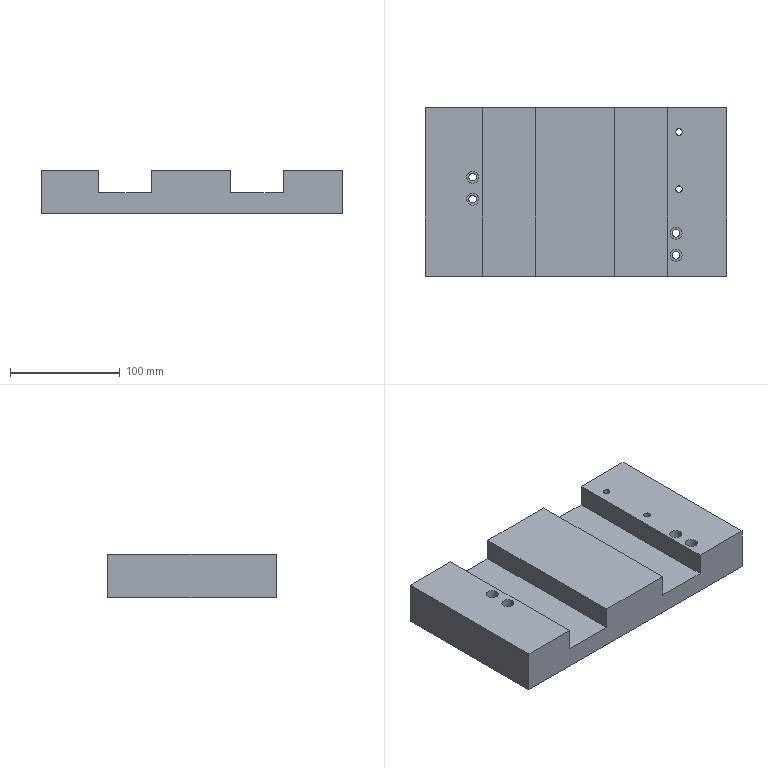Part | 1 solid | 38 faces | box 273.935 x 153 x 40 mm | volume 1364828 mm3 | cylinder 20 | plane 18 | commonest cylinder face diameters 7 x8 11 x8 6 x4